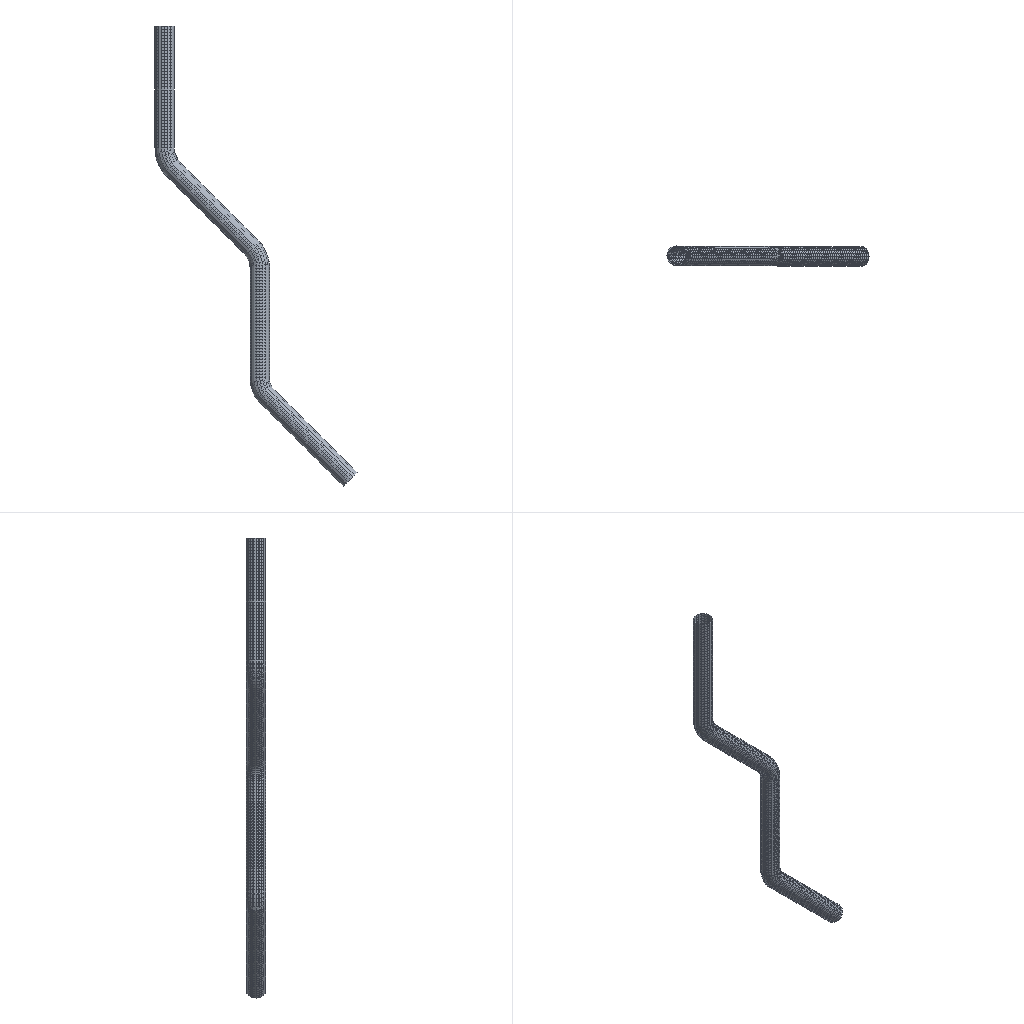Simulation study | abaqus
Set-up summary:
category,name,step,type,value,unit,region
solver,abaqus
solver,version,,,Abaqus/Standard 2020
units,not stated in the deck,,not stated
analysis,deck,,static,static
load_step,Step-1,Step-1,static
load_step,requested,,,1
mesh,nodes,,,6960
mesh,elements,,,3460
element_type,C3D8R,,solid,3460
load,load commands in deck,,count,1
bc,support commands in deck,,count,1
material,MATERIAL-1,,in results
check,setup vs results,,match,"per instance, exact: element labels, types and connectivity; labels of the nodes the elements use; coordinates of those nodes at SINGLE_PRECISION in 1 of 1 instance(s)"
Abaqus input file, long lists of numbers shortened:
*Heading
** Job name: Job-1 Model name: Model-1
** Generated by: Abaqus/CAE 2020
*Preprint, echo=NO, model=NO, history=NO, contact=NO
**
** PARTS
**
*Part, name=P45
*Node
      1,   295.033,   -9.405,  -600.946
      2,   297.536,   -12.944,  -598.443
** (6958 more lines like these left out)
*Element, type=C3D8R
   1,   59,   77,   69,   47,   19,   37,   29,    7
   2,   60,   48,   69,   77,   20,    8,   29,   37
** (3458 more lines like these left out)
*Nset, nset=Set-3, generate
    1,  6960,     1
*Elset, elset=Set-3, generate
    1,  3460,     1
** Section: Section-1
*Solid Section, elset=Set-3, material=Material-1
,
*End Part
**
**
** ASSEMBLY
**
*Assembly, name=Assembly
**
*Instance, name=P45-1, part=P45
*End Instance
**
*Nset, nset=Set-1, instance=P45-1
    1,    2,    3,    4,    5,    6,    7,    8,    9,   10,   11,   12,   13,   14,   15,   16
   17,   18,   19,   20,   21,   22,   23,   24,   25,   26,   27,   28,   29,   30,   31,   32
** (3 more lines like these left out)
*Elset, elset=Set-1, instance=P45-1
    1,    2,    3,    4,    5,    6,    7,    8,    9,   10,   11,   12,   13,   14,   15,   16
   17,   18,   19,   20, 3441, 3442, 3443, 3444, 3445, 3446, 3447, 3448, 3449, 3450, 3451, 3452
** (1 more lines like these left out)
*Elset, elset=_Surf-1_S3, internal, instance=P45-1
    1,    4,    6,    9,   10,   13,   15,   16,   19,   21,   24,   26,   29,   30,   33,   35
   36,   39,   41,   44,   46,   49,   50,   53,   55,   56,   59,   61,   64,   66,   69,   70
** (96 more lines like these left out)
*Elset, elset=_Surf-1_S6, internal, instance=P45-1
    2,    5,    7,   11,   12,   14,   17,   20,   22,   25,   27,   31,   32,   34,   37,   40
   42,   45,   47,   51,   52,   54,   57,   60,   62,   65,   67,   71,   72,   74,   77,   80
** (85 more lines like these left out)
*Elset, elset=_Surf-1_S4, internal, instance=P45-1, generate
    8,  3458,    10
*Elset, elset=_Surf-1_S5, internal, instance=P45-1, generate
    3,  3443,    20
*Surface, type=ELEMENT, name=Surf-1
_Surf-1_S3, S3
_Surf-1_S6, S6
_Surf-1_S4, S4
_Surf-1_S5, S5
*End Assembly
*Amplitude, name=Amp-1
             0.,              0.,              1.,              1.
**
** MATERIALS
**
*Material, name=Material-1
*Density
 7.8e-09,
*Elastic
210000., 0.3
*Plastic
350.,0.
** ----------------------------------------------------------------
**
** STEP: Step-1
**
*Step, name=Step-1, nlgeom=YES, inc=1000
*Static, stabilize=0.0002, allsdtol=0.05, continue=NO
0.01, 1., 1e-05, 1.
**
** BOUNDARY CONDITIONS
**
** Name: BC-1 Type: 对称/反对称/完全固定
*Boundary
Set-1, ENCASTRE
**
** LOADS
**
** Name: Load-1   Type: Pressure
*Dsload, amplitude=Amp-1
Surf-1, P, 0.24
**
** OUTPUT REQUESTS
**
*Restart, write, frequency=0
**
** FIELD OUTPUT: F-Output-1
**
*Output, field, variable=PRESELECT
**
** HISTORY OUTPUT: H-Output-1
**
*Output, history, variable=PRESELECT
*End Step
Results summary:
result,step,,completed,increments=11 time=1.0/1.0
result,analysis,,,static
result,last_loadstep,,,1
result,primary field,,,U
result,reaction total,,FX,117.997,model units
result,reaction total,,FY,-0.0,model units
result,reaction total,,FZ,48.876,model units